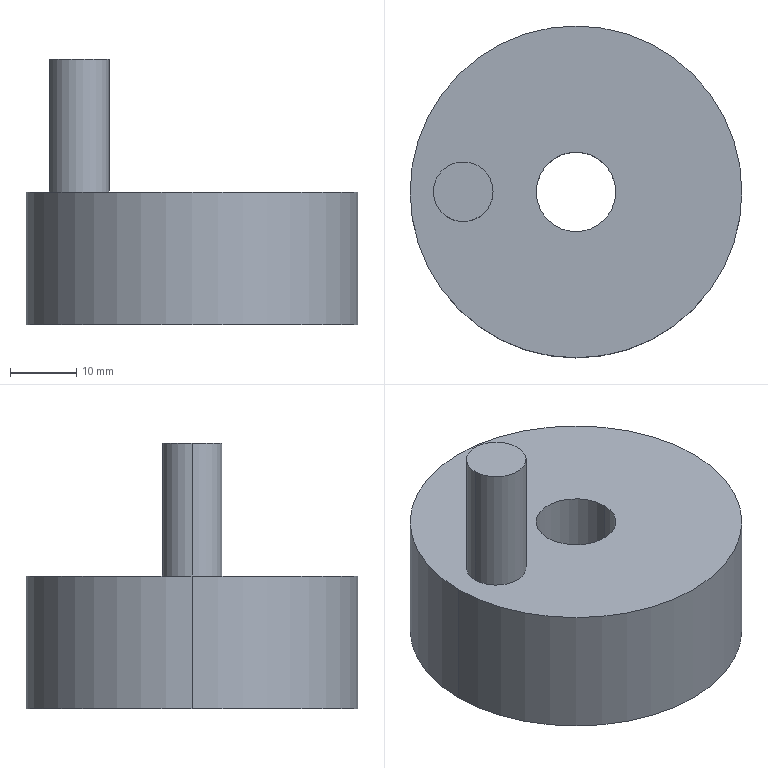Part | STEP file | MYT-A01-P17 | 1 solid | 9 faces | box 50 x 50 x 40 mm | volume 38280 mm3 | cylinder 6 | plane 3 | commonest cylinder face diameters 9 x2 12 x2 50 x2
STEP:
#1=CARTESIAN_POINT('',(-12.5,0.,40.));
#2=VERTEX_POINT('',#1);
#3=CARTESIAN_POINT('',(-21.5,0.,40.));
#4=VERTEX_POINT('',#3);
#5=CARTESIAN_POINT('',(-17.,0.,40.));
#6=DIRECTION('',(0.,0.,1.));
#7=DIRECTION('',(1.,0.,0.));
#8=AXIS2_PLACEMENT_3D('',#5,#6,#7);
#9=CIRCLE('',#8,4.5);
#10=EDGE_CURVE('',#2,#4,#9,.T.);
#11=ORIENTED_EDGE('',*,*,#10,.F.);
#12=CARTESIAN_POINT('',(-12.5,0.,20.));
#13=VERTEX_POINT('',#12);
#14=CARTESIAN_POINT('',(-12.5,0.,40.));
#15=DIRECTION('',(0.,0.,-1.));
#16=VECTOR('',#15,1000.);
#17=LINE('',#14,#16);
#18=EDGE_CURVE('',#2,#13,#17,.T.);
#19=ORIENTED_EDGE('',*,*,#18,.T.);
#20=CARTESIAN_POINT('',(-21.5,0.,20.));
#21=VERTEX_POINT('',#20);
#22=CARTESIAN_POINT('',(-17.,0.,20.));
#23=DIRECTION('',(0.,0.,1.));
#24=DIRECTION('',(1.,0.,0.));
#25=AXIS2_PLACEMENT_3D('',#22,#23,#24);
#26=CIRCLE('',#25,4.5);
#27=EDGE_CURVE('',#13,#21,#26,.T.);
#28=ORIENTED_EDGE('',*,*,#27,.T.);
#29=CARTESIAN_POINT('',(-21.5,0.,40.));
#30=DIRECTION('',(0.,0.,-1.));
#31=VECTOR('',#30,1000.);
#32=LINE('',#29,#31);
#33=EDGE_CURVE('',#4,#21,#32,.T.);
#34=ORIENTED_EDGE('',*,*,#33,.F.);
#35=EDGE_LOOP('',(#11,#19,#28,#34));
#36=FACE_OUTER_BOUND('',#35,.T.);
#37=CARTESIAN_POINT('',(-17.,0.,40.));
#38=DIRECTION('',(0.,0.,-1.));
#39=DIRECTION('',(-1.,0.,0.));
#40=AXIS2_PLACEMENT_3D('',#37,#38,#39);
#41=CYLINDRICAL_SURFACE('',#40,4.5);
#42=ADVANCED_FACE('',(#36),#41,.T.);
#43=CARTESIAN_POINT('',(-6.,0.,0.));
#44=VERTEX_POINT('',#43);
#45=CARTESIAN_POINT('',(6.,0.,0.));
#46=VERTEX_POINT('',#45);
#47=CARTESIAN_POINT('',(0.,0.,0.));
#48=DIRECTION('',(0.,0.,1.));
#49=DIRECTION('',(1.,0.,0.));
#50=AXIS2_PLACEMENT_3D('',#47,#48,#49);
#51=CIRCLE('',#50,6.);
#52=EDGE_CURVE('',#44,#46,#51,.T.);
#53=ORIENTED_EDGE('',*,*,#52,.F.);
#54=CARTESIAN_POINT('',(-6.,0.,20.));
#55=VERTEX_POINT('',#54);
#56=CARTESIAN_POINT('',(-6.,0.,0.));
#57=DIRECTION('',(0.,0.,1.));
#58=VECTOR('',#57,1000.);
#59=LINE('',#56,#58);
#60=EDGE_CURVE('',#44,#55,#59,.T.);
#61=ORIENTED_EDGE('',*,*,#60,.T.);
#62=CARTESIAN_POINT('',(6.,0.,20.));
#63=VERTEX_POINT('',#62);
#64=CARTESIAN_POINT('',(0.,0.,20.));
#65=DIRECTION('',(0.,0.,1.));
#66=DIRECTION('',(1.,0.,0.));
#67=AXIS2_PLACEMENT_3D('',#64,#65,#66);
#68=CIRCLE('',#67,6.);
#69=EDGE_CURVE('',#55,#63,#68,.T.);
#70=ORIENTED_EDGE('',*,*,#69,.T.);
#71=CARTESIAN_POINT('',(6.,0.,0.));
#72=DIRECTION('',(0.,0.,1.));
#73=VECTOR('',#72,1000.);
#74=LINE('',#71,#73);
#75=EDGE_CURVE('',#46,#63,#74,.T.);
#76=ORIENTED_EDGE('',*,*,#75,.F.);
#77=EDGE_LOOP('',(#53,#61,#70,#76));
#78=FACE_OUTER_BOUND('',#77,.T.);
#79=CARTESIAN_POINT('',(0.,0.,0.));
#80=DIRECTION('',(0.,0.,1.));
#81=DIRECTION('',(1.,0.,0.));
#82=AXIS2_PLACEMENT_3D('',#79,#80,#81);
#83=CYLINDRICAL_SURFACE('',#82,6.);
#84=ADVANCED_FACE('',(#78),#83,.F.);
#85=CARTESIAN_POINT('',(25.,0.,20.));
#86=VERTEX_POINT('',#85);
#87=CARTESIAN_POINT('',(-25.,0.,20.));
#88=VERTEX_POINT('',#87);
#89=CARTESIAN_POINT('',(0.,0.,20.));
#90=DIRECTION('',(0.,0.,1.));
#91=DIRECTION('',(1.,0.,0.));
#92=AXIS2_PLACEMENT_3D('',#89,#90,#91);
#93=CIRCLE('',#92,25.);
#94=EDGE_CURVE('',#86,#88,#93,.T.);
#95=ORIENTED_EDGE('',*,*,#94,.F.);
#96=CARTESIAN_POINT('',(25.,0.,0.));
#97=VERTEX_POINT('',#96);
#98=CARTESIAN_POINT('',(25.,0.,20.));
#99=DIRECTION('',(0.,0.,-1.));
#100=VECTOR('',#99,1000.);
#101=LINE('',#98,#100);
#102=EDGE_CURVE('',#86,#97,#101,.T.);
#103=ORIENTED_EDGE('',*,*,#102,.T.);
#104=CARTESIAN_POINT('',(-25.,0.,0.));
#105=VERTEX_POINT('',#104);
#106=CARTESIAN_POINT('',(0.,0.,0.));
#107=DIRECTION('',(0.,0.,1.));
#108=DIRECTION('',(1.,0.,0.));
#109=AXIS2_PLACEMENT_3D('',#106,#107,#108);
#110=CIRCLE('',#109,25.);
#111=EDGE_CURVE('',#97,#105,#110,.T.);
#112=ORIENTED_EDGE('',*,*,#111,.T.);
#113=CARTESIAN_POINT('',(-25.,0.,20.));
#114=DIRECTION('',(0.,0.,-1.));
#115=VECTOR('',#114,1000.);
#116=LINE('',#113,#115);
#117=EDGE_CURVE('',#88,#105,#116,.T.);
#118=ORIENTED_EDGE('',*,*,#117,.F.);
#119=EDGE_LOOP('',(#95,#103,#112,#118));
#120=FACE_OUTER_BOUND('',#119,.T.);
#121=CARTESIAN_POINT('',(0.,0.,20.));
#122=DIRECTION('',(0.,0.,-1.));
#123=DIRECTION('',(-1.,0.,0.));
#124=AXIS2_PLACEMENT_3D('',#121,#122,#123);
#125=CYLINDRICAL_SURFACE('',#124,25.);
#126=ADVANCED_FACE('',(#120),#125,.T.);
#127=ORIENTED_EDGE('',*,*,#102,.F.);
#128=CARTESIAN_POINT('',(0.,0.,20.));
#129=DIRECTION('',(0.,0.,1.));
#130=DIRECTION('',(1.,0.,0.));
#131=AXIS2_PLACEMENT_3D('',#128,#129,#130);
#132=CIRCLE('',#131,25.);
#133=EDGE_CURVE('',#88,#86,#132,.T.);
#134=ORIENTED_EDGE('',*,*,#133,.F.);
#135=ORIENTED_EDGE('',*,*,#117,.T.);
#136=CARTESIAN_POINT('',(0.,0.,0.));
#137=DIRECTION('',(0.,0.,1.));
#138=DIRECTION('',(1.,0.,0.));
#139=AXIS2_PLACEMENT_3D('',#136,#137,#138);
#140=CIRCLE('',#139,25.);
#141=EDGE_CURVE('',#105,#97,#140,.T.);
#142=ORIENTED_EDGE('',*,*,#141,.T.);
#143=EDGE_LOOP('',(#127,#134,#135,#142));
#144=FACE_OUTER_BOUND('',#143,.T.);
#145=CARTESIAN_POINT('',(0.,0.,20.));
#146=DIRECTION('',(0.,0.,-1.));
#147=DIRECTION('',(-1.,0.,0.));
#148=AXIS2_PLACEMENT_3D('',#145,#146,#147);
#149=CYLINDRICAL_SURFACE('',#148,25.);
#150=ADVANCED_FACE('',(#144),#149,.T.);
#151=CARTESIAN_POINT('',(-17.,0.,20.));
#152=DIRECTION('',(0.,0.,1.));
#153=DIRECTION('',(1.,0.,0.));
#154=AXIS2_PLACEMENT_3D('',#151,#152,#153);
#155=CIRCLE('',#154,4.5);
#156=EDGE_CURVE('',#21,#13,#155,.T.);
#157=ORIENTED_EDGE('',*,*,#156,.F.);
#158=ORIENTED_EDGE('',*,*,#27,.F.);
#159=EDGE_LOOP('',(#157,#158));
#160=FACE_BOUND('',#159,.T.);
#161=CARTESIAN_POINT('',(0.,0.,20.));
#162=DIRECTION('',(0.,0.,1.));
#163=DIRECTION('',(1.,0.,0.));
#164=AXIS2_PLACEMENT_3D('',#161,#162,#163);
#165=CIRCLE('',#164,6.);
#166=EDGE_CURVE('',#63,#55,#165,.T.);
#167=ORIENTED_EDGE('',*,*,#166,.F.);
#168=ORIENTED_EDGE('',*,*,#69,.F.);
#169=EDGE_LOOP('',(#167,#168));
#170=FACE_BOUND('',#169,.T.);
#171=ORIENTED_EDGE('',*,*,#133,.T.);
#172=ORIENTED_EDGE('',*,*,#94,.T.);
#173=EDGE_LOOP('',(#171,#172));
#174=FACE_OUTER_BOUND('',#173,.T.);
#175=CARTESIAN_POINT('',(0.,0.,20.));
#176=DIRECTION('',(0.,0.,1.));
#177=DIRECTION('',(1.,0.,0.));
#178=AXIS2_PLACEMENT_3D('',#175,#176,#177);
#179=PLANE('',#178);
#180=ADVANCED_FACE('',(#160,#170,#174),#179,.T.);
#181=CARTESIAN_POINT('',(0.,0.,0.));
#182=DIRECTION('',(0.,0.,1.));
#183=DIRECTION('',(1.,0.,0.));
#184=AXIS2_PLACEMENT_3D('',#181,#182,#183);
#185=CIRCLE('',#184,6.);
#186=EDGE_CURVE('',#46,#44,#185,.T.);
#187=ORIENTED_EDGE('',*,*,#186,.T.);
#188=ORIENTED_EDGE('',*,*,#52,.T.);
#189=EDGE_LOOP('',(#187,#188));
#190=FACE_BOUND('',#189,.T.);
#191=ORIENTED_EDGE('',*,*,#141,.F.);
#192=ORIENTED_EDGE('',*,*,#111,.F.);
#193=EDGE_LOOP('',(#191,#192));
#194=FACE_OUTER_BOUND('',#193,.T.);
#195=CARTESIAN_POINT('',(0.,0.,0.));
#196=DIRECTION('',(0.,0.,1.));
#197=DIRECTION('',(1.,0.,0.));
#198=AXIS2_PLACEMENT_3D('',#195,#196,#197);
#199=PLANE('',#198);
#200=ADVANCED_FACE('',(#190,#194),#199,.F.);
#201=ORIENTED_EDGE('',*,*,#60,.F.);
#202=ORIENTED_EDGE('',*,*,#186,.F.);
#203=ORIENTED_EDGE('',*,*,#75,.T.);
#204=ORIENTED_EDGE('',*,*,#166,.T.);
#205=EDGE_LOOP('',(#201,#202,#203,#204));
#206=FACE_OUTER_BOUND('',#205,.T.);
#207=CARTESIAN_POINT('',(0.,0.,0.));
#208=DIRECTION('',(0.,0.,1.));
#209=DIRECTION('',(1.,0.,0.));
#210=AXIS2_PLACEMENT_3D('',#207,#208,#209);
#211=CYLINDRICAL_SURFACE('',#210,6.);
#212=ADVANCED_FACE('',(#206),#211,.F.);
#213=ORIENTED_EDGE('',*,*,#18,.F.);
#214=CARTESIAN_POINT('',(-17.,0.,40.));
#215=DIRECTION('',(0.,0.,1.));
#216=DIRECTION('',(1.,0.,0.));
#217=AXIS2_PLACEMENT_3D('',#214,#215,#216);
#218=CIRCLE('',#217,4.5);
#219=EDGE_CURVE('',#4,#2,#218,.T.);
#220=ORIENTED_EDGE('',*,*,#219,.F.);
#221=ORIENTED_EDGE('',*,*,#33,.T.);
#222=ORIENTED_EDGE('',*,*,#156,.T.);
#223=EDGE_LOOP('',(#213,#220,#221,#222));
#224=FACE_OUTER_BOUND('',#223,.T.);
#225=CARTESIAN_POINT('',(-17.,0.,40.));
#226=DIRECTION('',(0.,0.,-1.));
#227=DIRECTION('',(-1.,0.,0.));
#228=AXIS2_PLACEMENT_3D('',#225,#226,#227);
#229=CYLINDRICAL_SURFACE('',#228,4.5);
#230=ADVANCED_FACE('',(#224),#229,.T.);
#231=ORIENTED_EDGE('',*,*,#219,.T.);
#232=ORIENTED_EDGE('',*,*,#10,.T.);
#233=EDGE_LOOP('',(#231,#232));
#234=FACE_OUTER_BOUND('',#233,.T.);
#235=CARTESIAN_POINT('',(-17.,0.,40.));
#236=DIRECTION('',(0.,0.,1.));
#237=DIRECTION('',(1.,0.,0.));
#238=AXIS2_PLACEMENT_3D('',#235,#236,#237);
#239=PLANE('',#238);
#240=ADVANCED_FACE('',(#234),#239,.T.);
#241=CLOSED_SHELL('',(#42,#84,#126,#150,#180,#200,#212,#230,#240));
#242=MANIFOLD_SOLID_BREP('',#241);
#243=CARTESIAN_POINT('',(0.,0.,0.));
#244=DIRECTION('',(0.,0.,1.));
#245=DIRECTION('',(1.,0.,0.));
#246=AXIS2_PLACEMENT_3D('',#243,#244,#245);
#247=(LENGTH_UNIT()NAMED_UNIT(*)SI_UNIT(.MILLI.,.METRE.));
#248=UNCERTAINTY_MEASURE_WITH_UNIT(LENGTH_MEASURE(0.00001),#247,'','');
#249=(NAMED_UNIT(*)PLANE_ANGLE_UNIT()SI_UNIT($,.RADIAN.));
#250=(NAMED_UNIT(*)SI_UNIT($,.STERADIAN.)SOLID_ANGLE_UNIT());
#251=(GEOMETRIC_REPRESENTATION_CONTEXT(3)GLOBAL_UNCERTAINTY_ASSIGNED_CONTEXT((#248))GLOBAL_UNIT_ASSIGNED_CONTEXT((#247,#249,#250))REPRESENTATION_CONTEXT('',''));
#252=ADVANCED_BREP_SHAPE_REPRESENTATION('',(#242,#246),#251);